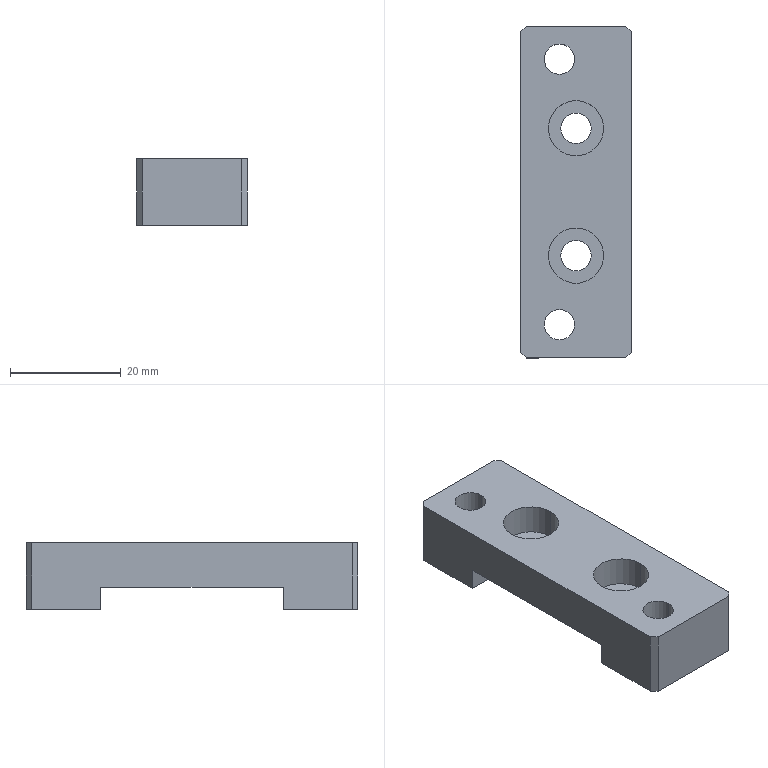Part | SolidWorks | features BaseBody 1 | 1 solid | 34 faces | box 20 x 60 x 12 mm | volume 9580 mm3 | plane 18 | cylinder 16 | commonest cylinder face diameters 5.5 x8 10 x8
STEP:
#1=CARTESIAN_POINT('',(93.009,112.551,12.));
#2=VERTEX_POINT('',#1);
#3=CARTESIAN_POINT('',(87.509,112.551,12.));
#4=VERTEX_POINT('',#3);
#5=CARTESIAN_POINT('',(90.259,112.551,12.));
#6=DIRECTION('',(0.,0.,-1.));
#7=DIRECTION('',(-1.,0.,0.));
#8=AXIS2_PLACEMENT_3D('',#5,#6,#7);
#9=CIRCLE('',#8,2.75);
#10=EDGE_CURVE('',#2,#4,#9,.T.);
#11=ORIENTED_EDGE('',*,*,#10,.F.);
#12=CARTESIAN_POINT('',(93.009,112.551,5.5));
#13=VERTEX_POINT('',#12);
#14=CARTESIAN_POINT('',(93.009,112.551,64.374));
#15=DIRECTION('',(0.,0.,-1.));
#16=VECTOR('',#15,1000.);
#17=LINE('',#14,#16);
#18=EDGE_CURVE('',#2,#13,#17,.T.);
#19=ORIENTED_EDGE('',*,*,#18,.T.);
#20=CARTESIAN_POINT('',(87.509,112.551,5.5));
#21=VERTEX_POINT('',#20);
#22=CARTESIAN_POINT('',(90.259,112.551,5.5));
#23=DIRECTION('',(0.,0.,1.));
#24=DIRECTION('',(-1.,0.,0.));
#25=AXIS2_PLACEMENT_3D('',#22,#23,#24);
#26=CIRCLE('',#25,2.75);
#27=EDGE_CURVE('',#21,#13,#26,.T.);
#28=ORIENTED_EDGE('',*,*,#27,.F.);
#29=CARTESIAN_POINT('',(87.509,112.551,64.374));
#30=DIRECTION('',(0.,0.,-1.));
#31=VECTOR('',#30,1000.);
#32=LINE('',#29,#31);
#33=EDGE_CURVE('',#4,#21,#32,.T.);
#34=ORIENTED_EDGE('',*,*,#33,.F.);
#35=EDGE_LOOP('',(#11,#19,#28,#34));
#36=FACE_OUTER_BOUND('',#35,.T.);
#37=CARTESIAN_POINT('',(90.259,112.551,64.374));
#38=DIRECTION('',(0.,0.,-1.));
#39=DIRECTION('',(-1.,0.,0.));
#40=AXIS2_PLACEMENT_3D('',#37,#38,#39);
#41=CYLINDRICAL_SURFACE('',#40,2.75);
#42=ADVANCED_FACE('',(#36),#41,.F.);
#43=CARTESIAN_POINT('',(93.009,64.551,12.));
#44=VERTEX_POINT('',#43);
#45=CARTESIAN_POINT('',(87.509,64.551,12.));
#46=VERTEX_POINT('',#45);
#47=CARTESIAN_POINT('',(90.259,64.551,12.));
#48=DIRECTION('',(0.,0.,-1.));
#49=DIRECTION('',(-1.,0.,0.));
#50=AXIS2_PLACEMENT_3D('',#47,#48,#49);
#51=CIRCLE('',#50,2.75);
#52=EDGE_CURVE('',#44,#46,#51,.T.);
#53=ORIENTED_EDGE('',*,*,#52,.F.);
#54=CARTESIAN_POINT('',(93.009,64.551,5.5));
#55=VERTEX_POINT('',#54);
#56=CARTESIAN_POINT('',(93.009,64.551,64.374));
#57=DIRECTION('',(0.,0.,-1.));
#58=VECTOR('',#57,1000.);
#59=LINE('',#56,#58);
#60=EDGE_CURVE('',#44,#55,#59,.T.);
#61=ORIENTED_EDGE('',*,*,#60,.T.);
#62=CARTESIAN_POINT('',(87.509,64.551,5.5));
#63=VERTEX_POINT('',#62);
#64=CARTESIAN_POINT('',(90.259,64.551,5.5));
#65=DIRECTION('',(0.,0.,1.));
#66=DIRECTION('',(-1.,0.,0.));
#67=AXIS2_PLACEMENT_3D('',#64,#65,#66);
#68=CIRCLE('',#67,2.75);
#69=EDGE_CURVE('',#63,#55,#68,.T.);
#70=ORIENTED_EDGE('',*,*,#69,.F.);
#71=CARTESIAN_POINT('',(87.509,64.551,64.374));
#72=DIRECTION('',(0.,0.,-1.));
#73=VECTOR('',#72,1000.);
#74=LINE('',#71,#73);
#75=EDGE_CURVE('',#46,#63,#74,.T.);
#76=ORIENTED_EDGE('',*,*,#75,.F.);
#77=EDGE_LOOP('',(#53,#61,#70,#76));
#78=FACE_OUTER_BOUND('',#77,.T.);
#79=CARTESIAN_POINT('',(90.259,64.551,64.374));
#80=DIRECTION('',(0.,0.,-1.));
#81=DIRECTION('',(-1.,0.,0.));
#82=AXIS2_PLACEMENT_3D('',#79,#80,#81);
#83=CYLINDRICAL_SURFACE('',#82,2.75);
#84=ADVANCED_FACE('',(#78),#83,.F.);
#85=CARTESIAN_POINT('',(88.259,100.051,6.5));
#86=VERTEX_POINT('',#85);
#87=CARTESIAN_POINT('',(98.259,100.051,6.5));
#88=VERTEX_POINT('',#87);
#89=CARTESIAN_POINT('',(93.259,100.051,6.5));
#90=DIRECTION('',(0.,0.,1.));
#91=DIRECTION('',(1.,0.,0.));
#92=AXIS2_PLACEMENT_3D('',#89,#90,#91);
#93=CIRCLE('',#92,5.);
#94=EDGE_CURVE('',#86,#88,#93,.T.);
#95=ORIENTED_EDGE('',*,*,#94,.F.);
#96=CARTESIAN_POINT('',(88.259,100.051,12.));
#97=VERTEX_POINT('',#96);
#98=CARTESIAN_POINT('',(88.259,100.051,9.25));
#99=DIRECTION('',(0.,0.,1.));
#100=VECTOR('',#99,1000.);
#101=LINE('',#98,#100);
#102=EDGE_CURVE('',#86,#97,#101,.T.);
#103=ORIENTED_EDGE('',*,*,#102,.T.);
#104=CARTESIAN_POINT('',(98.259,100.051,12.));
#105=VERTEX_POINT('',#104);
#106=CARTESIAN_POINT('',(93.259,100.051,12.));
#107=DIRECTION('',(0.,0.,-1.));
#108=DIRECTION('',(1.,0.,0.));
#109=AXIS2_PLACEMENT_3D('',#106,#107,#108);
#110=CIRCLE('',#109,5.);
#111=EDGE_CURVE('',#105,#97,#110,.T.);
#112=ORIENTED_EDGE('',*,*,#111,.F.);
#113=CARTESIAN_POINT('',(98.259,100.051,9.25));
#114=DIRECTION('',(0.,0.,1.));
#115=VECTOR('',#114,1000.);
#116=LINE('',#113,#115);
#117=EDGE_CURVE('',#88,#105,#116,.T.);
#118=ORIENTED_EDGE('',*,*,#117,.F.);
#119=EDGE_LOOP('',(#95,#103,#112,#118));
#120=FACE_OUTER_BOUND('',#119,.T.);
#121=CARTESIAN_POINT('',(93.259,100.051,9.25));
#122=DIRECTION('',(0.,0.,1.));
#123=DIRECTION('',(1.,0.,0.));
#124=AXIS2_PLACEMENT_3D('',#121,#122,#123);
#125=CYLINDRICAL_SURFACE('',#124,5.);
#126=ADVANCED_FACE('',(#120),#125,.F.);
#127=CARTESIAN_POINT('',(88.259,77.051,6.5));
#128=VERTEX_POINT('',#127);
#129=CARTESIAN_POINT('',(98.259,77.051,6.5));
#130=VERTEX_POINT('',#129);
#131=CARTESIAN_POINT('',(93.259,77.051,6.5));
#132=DIRECTION('',(0.,0.,1.));
#133=DIRECTION('',(1.,0.,0.));
#134=AXIS2_PLACEMENT_3D('',#131,#132,#133);
#135=CIRCLE('',#134,5.);
#136=EDGE_CURVE('',#128,#130,#135,.T.);
#137=ORIENTED_EDGE('',*,*,#136,.F.);
#138=CARTESIAN_POINT('',(88.259,77.051,12.));
#139=VERTEX_POINT('',#138);
#140=CARTESIAN_POINT('',(88.259,77.051,9.25));
#141=DIRECTION('',(0.,0.,1.));
#142=VECTOR('',#141,1000.);
#143=LINE('',#140,#142);
#144=EDGE_CURVE('',#128,#139,#143,.T.);
#145=ORIENTED_EDGE('',*,*,#144,.T.);
#146=CARTESIAN_POINT('',(98.259,77.051,12.));
#147=VERTEX_POINT('',#146);
#148=CARTESIAN_POINT('',(93.259,77.051,12.));
#149=DIRECTION('',(0.,0.,-1.));
#150=DIRECTION('',(1.,0.,0.));
#151=AXIS2_PLACEMENT_3D('',#148,#149,#150);
#152=CIRCLE('',#151,5.);
#153=EDGE_CURVE('',#147,#139,#152,.T.);
#154=ORIENTED_EDGE('',*,*,#153,.F.);
#155=CARTESIAN_POINT('',(98.259,77.051,9.25));
#156=DIRECTION('',(0.,0.,1.));
#157=VECTOR('',#156,1000.);
#158=LINE('',#155,#157);
#159=EDGE_CURVE('',#130,#147,#158,.T.);
#160=ORIENTED_EDGE('',*,*,#159,.F.);
#161=EDGE_LOOP('',(#137,#145,#154,#160));
#162=FACE_OUTER_BOUND('',#161,.T.);
#163=CARTESIAN_POINT('',(93.259,77.051,9.25));
#164=DIRECTION('',(0.,0.,1.));
#165=DIRECTION('',(1.,0.,0.));
#166=AXIS2_PLACEMENT_3D('',#163,#164,#165);
#167=CYLINDRICAL_SURFACE('',#166,5.);
#168=ADVANCED_FACE('',(#162),#167,.F.);
#169=CARTESIAN_POINT('',(95.259,112.551,5.5));
#170=VERTEX_POINT('',#169);
#171=CARTESIAN_POINT('',(85.259,112.551,5.5));
#172=VERTEX_POINT('',#171);
#173=CARTESIAN_POINT('',(90.259,112.551,5.5));
#174=DIRECTION('',(0.,0.,-1.));
#175=DIRECTION('',(-1.,0.,0.));
#176=AXIS2_PLACEMENT_3D('',#173,#174,#175);
#177=CIRCLE('',#176,5.);
#178=EDGE_CURVE('',#170,#172,#177,.T.);
#179=ORIENTED_EDGE('',*,*,#178,.F.);
#180=CARTESIAN_POINT('',(95.259,112.551,0.));
#181=VERTEX_POINT('',#180);
#182=CARTESIAN_POINT('',(95.259,112.551,2.75));
#183=DIRECTION('',(0.,0.,-1.));
#184=VECTOR('',#183,1000.);
#185=LINE('',#182,#184);
#186=EDGE_CURVE('',#170,#181,#185,.T.);
#187=ORIENTED_EDGE('',*,*,#186,.T.);
#188=CARTESIAN_POINT('',(85.259,112.551,0.));
#189=VERTEX_POINT('',#188);
#190=CARTESIAN_POINT('',(90.259,112.551,0.));
#191=DIRECTION('',(0.,0.,-1.));
#192=DIRECTION('',(-1.,0.,0.));
#193=AXIS2_PLACEMENT_3D('',#190,#191,#192);
#194=CIRCLE('',#193,5.);
#195=EDGE_CURVE('',#181,#189,#194,.T.);
#196=ORIENTED_EDGE('',*,*,#195,.T.);
#197=CARTESIAN_POINT('',(85.259,112.551,2.75));
#198=DIRECTION('',(0.,0.,-1.));
#199=VECTOR('',#198,1000.);
#200=LINE('',#197,#199);
#201=EDGE_CURVE('',#172,#189,#200,.T.);
#202=ORIENTED_EDGE('',*,*,#201,.F.);
#203=EDGE_LOOP('',(#179,#187,#196,#202));
#204=FACE_OUTER_BOUND('',#203,.T.);
#205=CARTESIAN_POINT('',(90.259,112.551,2.75));
#206=DIRECTION('',(0.,0.,-1.));
#207=DIRECTION('',(-1.,0.,0.));
#208=AXIS2_PLACEMENT_3D('',#205,#206,#207);
#209=CYLINDRICAL_SURFACE('',#208,5.);
#210=ADVANCED_FACE('',(#204),#209,.F.);
#211=CARTESIAN_POINT('',(95.259,64.551,5.5));
#212=VERTEX_POINT('',#211);
#213=CARTESIAN_POINT('',(85.259,64.551,5.5));
#214=VERTEX_POINT('',#213);
#215=CARTESIAN_POINT('',(90.259,64.551,5.5));
#216=DIRECTION('',(0.,0.,-1.));
#217=DIRECTION('',(-1.,0.,0.));
#218=AXIS2_PLACEMENT_3D('',#215,#216,#217);
#219=CIRCLE('',#218,5.);
#220=EDGE_CURVE('',#212,#214,#219,.T.);
#221=ORIENTED_EDGE('',*,*,#220,.F.);
#222=CARTESIAN_POINT('',(95.259,64.551,0.));
#223=VERTEX_POINT('',#222);
#224=CARTESIAN_POINT('',(95.259,64.551,2.75));
#225=DIRECTION('',(0.,0.,-1.));
#226=VECTOR('',#225,1000.);
#227=LINE('',#224,#226);
#228=EDGE_CURVE('',#212,#223,#227,.T.);
#229=ORIENTED_EDGE('',*,*,#228,.T.);
#230=CARTESIAN_POINT('',(85.259,64.551,0.));
#231=VERTEX_POINT('',#230);
#232=CARTESIAN_POINT('',(90.259,64.551,0.));
#233=DIRECTION('',(0.,0.,-1.));
#234=DIRECTION('',(-1.,0.,0.));
#235=AXIS2_PLACEMENT_3D('',#232,#233,#234);
#236=CIRCLE('',#235,5.);
#237=EDGE_CURVE('',#223,#231,#236,.T.);
#238=ORIENTED_EDGE('',*,*,#237,.T.);
#239=CARTESIAN_POINT('',(85.259,64.551,2.75));
#240=DIRECTION('',(0.,0.,-1.));
#241=VECTOR('',#240,1000.);
#242=LINE('',#239,#241);
#243=EDGE_CURVE('',#214,#231,#242,.T.);
#244=ORIENTED_EDGE('',*,*,#243,.F.);
#245=EDGE_LOOP('',(#221,#229,#238,#244));
#246=FACE_OUTER_BOUND('',#245,.T.);
#247=CARTESIAN_POINT('',(90.259,64.551,2.75));
#248=DIRECTION('',(0.,0.,-1.));
#249=DIRECTION('',(-1.,0.,0.));
#250=AXIS2_PLACEMENT_3D('',#247,#248,#249);
#251=CYLINDRICAL_SURFACE('',#250,5.);
#252=ADVANCED_FACE('',(#246),#251,.F.);
#253=CARTESIAN_POINT('',(96.009,100.051,4.));
#254=VERTEX_POINT('',#253);
#255=CARTESIAN_POINT('',(90.509,100.051,4.));
#256=VERTEX_POINT('',#255);
#257=CARTESIAN_POINT('',(93.259,100.051,4.));
#258=DIRECTION('',(0.,0.,-1.));
#259=DIRECTION('',(1.,0.,0.));
#260=AXIS2_PLACEMENT_3D('',#257,#258,#259);
#261=CIRCLE('',#260,2.75);
#262=EDGE_CURVE('',#254,#256,#261,.T.);
#263=ORIENTED_EDGE('',*,*,#262,.T.);
#264=CARTESIAN_POINT('',(90.509,100.051,6.5));
#265=VERTEX_POINT('',#264);
#266=CARTESIAN_POINT('',(90.509,100.051,-52.374));
#267=DIRECTION('',(0.,0.,1.));
#268=VECTOR('',#267,1000.);
#269=LINE('',#266,#268);
#270=EDGE_CURVE('',#256,#265,#269,.T.);
#271=ORIENTED_EDGE('',*,*,#270,.T.);
#272=CARTESIAN_POINT('',(96.009,100.051,6.5));
#273=VERTEX_POINT('',#272);
#274=CARTESIAN_POINT('',(93.259,100.051,6.5));
#275=DIRECTION('',(0.,0.,-1.));
#276=DIRECTION('',(1.,0.,0.));
#277=AXIS2_PLACEMENT_3D('',#274,#275,#276);
#278=CIRCLE('',#277,2.75);
#279=EDGE_CURVE('',#273,#265,#278,.T.);
#280=ORIENTED_EDGE('',*,*,#279,.F.);
#281=CARTESIAN_POINT('',(96.009,100.051,-52.374));
#282=DIRECTION('',(0.,0.,1.));
#283=VECTOR('',#282,1000.);
#284=LINE('',#281,#283);
#285=EDGE_CURVE('',#254,#273,#284,.T.);
#286=ORIENTED_EDGE('',*,*,#285,.F.);
#287=EDGE_LOOP('',(#263,#271,#280,#286));
#288=FACE_OUTER_BOUND('',#287,.T.);
#289=CARTESIAN_POINT('',(93.259,100.051,-52.374));
#290=DIRECTION('',(0.,0.,1.));
#291=DIRECTION('',(1.,0.,0.));
#292=AXIS2_PLACEMENT_3D('',#289,#290,#291);
#293=CYLINDRICAL_SURFACE('',#292,2.75);
#294=ADVANCED_FACE('',(#288),#293,.F.);
#295=CARTESIAN_POINT('',(96.009,77.051,4.));
#296=VERTEX_POINT('',#295);
#297=CARTESIAN_POINT('',(90.509,77.051,4.));
#298=VERTEX_POINT('',#297);
#299=CARTESIAN_POINT('',(93.259,77.051,4.));
#300=DIRECTION('',(0.,0.,-1.));
#301=DIRECTION('',(1.,0.,0.));
#302=AXIS2_PLACEMENT_3D('',#299,#300,#301);
#303=CIRCLE('',#302,2.75);
#304=EDGE_CURVE('',#296,#298,#303,.T.);
#305=ORIENTED_EDGE('',*,*,#304,.T.);
#306=CARTESIAN_POINT('',(90.509,77.051,6.5));
#307=VERTEX_POINT('',#306);
#308=CARTESIAN_POINT('',(90.509,77.051,-52.374));
#309=DIRECTION('',(0.,0.,1.));
#310=VECTOR('',#309,1000.);
#311=LINE('',#308,#310);
#312=EDGE_CURVE('',#298,#307,#311,.T.);
#313=ORIENTED_EDGE('',*,*,#312,.T.);
#314=CARTESIAN_POINT('',(96.009,77.051,6.5));
#315=VERTEX_POINT('',#314);
#316=CARTESIAN_POINT('',(93.259,77.051,6.5));
#317=DIRECTION('',(0.,0.,-1.));
#318=DIRECTION('',(1.,0.,0.));
#319=AXIS2_PLACEMENT_3D('',#316,#317,#318);
#320=CIRCLE('',#319,2.75);
#321=EDGE_CURVE('',#315,#307,#320,.T.);
#322=ORIENTED_EDGE('',*,*,#321,.F.);
#323=CARTESIAN_POINT('',(96.009,77.051,-52.374));
#324=DIRECTION('',(0.,0.,1.));
#325=VECTOR('',#324,1000.);
#326=LINE('',#323,#325);
#327=EDGE_CURVE('',#296,#315,#326,.T.);
#328=ORIENTED_EDGE('',*,*,#327,.F.);
#329=EDGE_LOOP('',(#305,#313,#322,#328));
#330=FACE_OUTER_BOUND('',#329,.T.);
#331=CARTESIAN_POINT('',(93.259,77.051,-52.374));
#332=DIRECTION('',(0.,0.,1.));
#333=DIRECTION('',(1.,0.,0.));
#334=AXIS2_PLACEMENT_3D('',#331,#332,#333);
#335=CYLINDRICAL_SURFACE('',#334,2.75);
#336=ADVANCED_FACE('',(#330),#335,.F.);
#337=CARTESIAN_POINT('',(90.259,112.551,12.));
#338=DIRECTION('',(0.,0.,-1.));
#339=DIRECTION('',(-1.,0.,0.));
#340=AXIS2_PLACEMENT_3D('',#337,#338,#339);
#341=CIRCLE('',#340,2.75);
#342=EDGE_CURVE('',#4,#2,#341,.T.);
#343=ORIENTED_EDGE('',*,*,#342,.T.);
#344=ORIENTED_EDGE('',*,*,#10,.T.);
#345=EDGE_LOOP('',(#343,#344));
#346=FACE_BOUND('',#345,.T.);
#347=CARTESIAN_POINT('',(90.259,64.551,12.));
#348=DIRECTION('',(0.,0.,-1.));
#349=DIRECTION('',(-1.,0.,0.));
#350=AXIS2_PLACEMENT_3D('',#347,#348,#349);
#351=CIRCLE('',#350,2.75);
#352=EDGE_CURVE('',#46,#44,#351,.T.);
#353=ORIENTED_EDGE('',*,*,#352,.T.);
#354=ORIENTED_EDGE('',*,*,#52,.T.);
#355=EDGE_LOOP('',(#353,#354));
#356=FACE_BOUND('',#355,.T.);
#357=ORIENTED_EDGE('',*,*,#111,.T.);
#358=CARTESIAN_POINT('',(93.259,100.051,12.));
#359=DIRECTION('',(0.,0.,-1.));
#360=DIRECTION('',(1.,0.,0.));
#361=AXIS2_PLACEMENT_3D('',#358,#359,#360);
#362=CIRCLE('',#361,5.);
#363=EDGE_CURVE('',#97,#105,#362,.T.);
#364=ORIENTED_EDGE('',*,*,#363,.T.);
#365=EDGE_LOOP('',(#357,#364));
#366=FACE_BOUND('',#365,.T.);
#367=ORIENTED_EDGE('',*,*,#153,.T.);
#368=CARTESIAN_POINT('',(93.259,77.051,12.));
#369=DIRECTION('',(0.,0.,-1.));
#370=DIRECTION('',(1.,0.,0.));
#371=AXIS2_PLACEMENT_3D('',#368,#369,#370);
#372=CIRCLE('',#371,5.);
#373=EDGE_CURVE('',#139,#147,#372,.T.);
#374=ORIENTED_EDGE('',*,*,#373,.T.);
#375=EDGE_LOOP('',(#367,#374));
#376=FACE_BOUND('',#375,.T.);
#377=CARTESIAN_POINT('',(84.259,58.551,12.));
#378=VERTEX_POINT('',#377);
#379=CARTESIAN_POINT('',(83.259,59.551,12.));
#380=VERTEX_POINT('',#379);
#381=CARTESIAN_POINT('',(83.759,59.051,12.));
#382=DIRECTION('',(-0.7071,0.7071,0.));
#383=VECTOR('',#382,1000.);
#384=LINE('',#381,#383);
#385=EDGE_CURVE('',#378,#380,#384,.T.);
#386=ORIENTED_EDGE('',*,*,#385,.F.);
#387=CARTESIAN_POINT('',(102.259,58.551,12.));
#388=VERTEX_POINT('',#387);
#389=CARTESIAN_POINT('',(93.259,58.551,12.));
#390=DIRECTION('',(1.,0.,0.));
#391=VECTOR('',#390,1000.);
#392=LINE('',#389,#391);
#393=EDGE_CURVE('',#378,#388,#392,.T.);
#394=ORIENTED_EDGE('',*,*,#393,.T.);
#395=CARTESIAN_POINT('',(103.259,59.551,12.));
#396=VERTEX_POINT('',#395);
#397=CARTESIAN_POINT('',(102.759,59.051,12.));
#398=DIRECTION('',(-0.7071,-0.7071,0.));
#399=VECTOR('',#398,1000.);
#400=LINE('',#397,#399);
#401=EDGE_CURVE('',#396,#388,#400,.T.);
#402=ORIENTED_EDGE('',*,*,#401,.F.);
#403=CARTESIAN_POINT('',(103.259,117.551,12.));
#404=VERTEX_POINT('',#403);
#405=CARTESIAN_POINT('',(103.259,88.551,12.));
#406=DIRECTION('',(0.,1.,0.));
#407=VECTOR('',#406,1000.);
#408=LINE('',#405,#407);
#409=EDGE_CURVE('',#396,#404,#408,.T.);
#410=ORIENTED_EDGE('',*,*,#409,.T.);
#411=CARTESIAN_POINT('',(102.259,118.551,12.));
#412=VERTEX_POINT('',#411);
#413=CARTESIAN_POINT('',(102.759,118.051,12.));
#414=DIRECTION('',(0.7071,-0.7071,0.));
#415=VECTOR('',#414,1000.);
#416=LINE('',#413,#415);
#417=EDGE_CURVE('',#412,#404,#416,.T.);
#418=ORIENTED_EDGE('',*,*,#417,.F.);
#419=CARTESIAN_POINT('',(84.259,118.551,12.));
#420=VERTEX_POINT('',#419);
#421=CARTESIAN_POINT('',(93.259,118.551,12.));
#422=DIRECTION('',(-1.,0.,0.));
#423=VECTOR('',#422,1000.);
#424=LINE('',#421,#423);
#425=EDGE_CURVE('',#412,#420,#424,.T.);
#426=ORIENTED_EDGE('',*,*,#425,.T.);
#427=CARTESIAN_POINT('',(83.259,117.551,12.));
#428=VERTEX_POINT('',#427);
#429=CARTESIAN_POINT('',(83.759,118.051,12.));
#430=DIRECTION('',(0.7071,0.7071,0.));
#431=VECTOR('',#430,1000.);
#432=LINE('',#429,#431);
#433=EDGE_CURVE('',#428,#420,#432,.T.);
#434=ORIENTED_EDGE('',*,*,#433,.F.);
#435=CARTESIAN_POINT('',(83.259,88.551,12.));
#436=DIRECTION('',(0.,-1.,0.));
#437=VECTOR('',#436,1000.);
#438=LINE('',#435,#437);
#439=EDGE_CURVE('',#428,#380,#438,.T.);
#440=ORIENTED_EDGE('',*,*,#439,.T.);
#441=EDGE_LOOP('',(#386,#394,#402,#410,#418,#426,#434,#440));
#442=FACE_OUTER_BOUND('',#441,.T.);
#443=CARTESIAN_POINT('',(93.259,88.551,12.));
#444=DIRECTION('',(0.,0.,1.));
#445=DIRECTION('',(1.,0.,0.));
#446=AXIS2_PLACEMENT_3D('',#443,#444,#445);
#447=PLANE('',#446);
#448=ADVANCED_FACE('',(#346,#356,#366,#376,#442),#447,.T.);
#449=ORIENTED_EDGE('',*,*,#18,.F.);
#450=ORIENTED_EDGE('',*,*,#342,.F.);
#451=ORIENTED_EDGE('',*,*,#33,.T.);
#452=CARTESIAN_POINT('',(90.259,112.551,5.5));
#453=DIRECTION('',(0.,0.,1.));
#454=DIRECTION('',(-1.,0.,0.));
#455=AXIS2_PLACEMENT_3D('',#452,#453,#454);
#456=CIRCLE('',#455,2.75);
#457=EDGE_CURVE('',#13,#21,#456,.T.);
#458=ORIENTED_EDGE('',*,*,#457,.F.);
#459=EDGE_LOOP('',(#449,#450,#451,#458));
#460=FACE_OUTER_BOUND('',#459,.T.);
#461=CARTESIAN_POINT('',(90.259,112.551,64.374));
#462=DIRECTION('',(0.,0.,-1.));
#463=DIRECTION('',(-1.,0.,0.));
#464=AXIS2_PLACEMENT_3D('',#461,#462,#463);
#465=CYLINDRICAL_SURFACE('',#464,2.75);
#466=ADVANCED_FACE('',(#460),#465,.F.);
#467=ORIENTED_EDGE('',*,*,#60,.F.);
#468=ORIENTED_EDGE('',*,*,#352,.F.);
#469=ORIENTED_EDGE('',*,*,#75,.T.);
#470=CARTESIAN_POINT('',(90.259,64.551,5.5));
#471=DIRECTION('',(0.,0.,1.));
#472=DIRECTION('',(-1.,0.,0.));
#473=AXIS2_PLACEMENT_3D('',#470,#471,#472);
#474=CIRCLE('',#473,2.75);
#475=EDGE_CURVE('',#55,#63,#474,.T.);
#476=ORIENTED_EDGE('',*,*,#475,.F.);
#477=EDGE_LOOP('',(#467,#468,#469,#476));
#478=FACE_OUTER_BOUND('',#477,.T.);
#479=CARTESIAN_POINT('',(90.259,64.551,64.374));
#480=DIRECTION('',(0.,0.,-1.));
#481=DIRECTION('',(-1.,0.,0.));
#482=AXIS2_PLACEMENT_3D('',#479,#480,#481);
#483=CYLINDRICAL_SURFACE('',#482,2.75);
#484=ADVANCED_FACE('',(#478),#483,.F.);
#485=ORIENTED_EDGE('',*,*,#102,.F.);
#486=CARTESIAN_POINT('',(93.259,100.051,6.5));
#487=DIRECTION('',(0.,0.,1.));
#488=DIRECTION('',(1.,0.,0.));
#489=AXIS2_PLACEMENT_3D('',#486,#487,#488);
#490=CIRCLE('',#489,5.);
#491=EDGE_CURVE('',#88,#86,#490,.T.);
#492=ORIENTED_EDGE('',*,*,#491,.F.);
#493=ORIENTED_EDGE('',*,*,#117,.T.);
#494=ORIENTED_EDGE('',*,*,#363,.F.);
#495=EDGE_LOOP('',(#485,#492,#493,#494));
#496=FACE_OUTER_BOUND('',#495,.T.);
#497=CARTESIAN_POINT('',(93.259,100.051,9.25));
#498=DIRECTION('',(0.,0.,1.));
#499=DIRECTION('',(1.,0.,0.));
#500=AXIS2_PLACEMENT_3D('',#497,#498,#499);
#501=CYLINDRICAL_SURFACE('',#500,5.);
#502=ADVANCED_FACE('',(#496),#501,.F.);
#503=ORIENTED_EDGE('',*,*,#144,.F.);
#504=CARTESIAN_POINT('',(93.259,77.051,6.5));
#505=DIRECTION('',(0.,0.,1.));
#506=DIRECTION('',(1.,0.,0.));
#507=AXIS2_PLACEMENT_3D('',#504,#505,#506);
#508=CIRCLE('',#507,5.);
#509=EDGE_CURVE('',#130,#128,#508,.T.);
#510=ORIENTED_EDGE('',*,*,#509,.F.);
#511=ORIENTED_EDGE('',*,*,#159,.T.);
#512=ORIENTED_EDGE('',*,*,#373,.F.);
#513=EDGE_LOOP('',(#503,#510,#511,#512));
#514=FACE_OUTER_BOUND('',#513,.T.);
#515=CARTESIAN_POINT('',(93.259,77.051,9.25));
#516=DIRECTION('',(0.,0.,1.));
#517=DIRECTION('',(1.,0.,0.));
#518=AXIS2_PLACEMENT_3D('',#515,#516,#517);
#519=CYLINDRICAL_SURFACE('',#518,5.);
#520=ADVANCED_FACE('',(#514),#519,.F.);
#521=CARTESIAN_POINT('',(84.259,58.551,0.));
#522=VERTEX_POINT('',#521);
#523=CARTESIAN_POINT('',(84.259,58.551,0.));
#524=DIRECTION('',(0.,0.,-1.));
#525=VECTOR('',#524,1000.);
#526=LINE('',#523,#525);
#527=EDGE_CURVE('',#378,#522,#526,.T.);
#528=ORIENTED_EDGE('',*,*,#527,.T.);
#529=CARTESIAN_POINT('',(102.259,58.551,0.));
#530=VERTEX_POINT('',#529);
#531=CARTESIAN_POINT('',(103.259,58.551,0.));
#532=DIRECTION('',(1.,0.,0.));
#533=VECTOR('',#532,1000.);
#534=LINE('',#531,#533);
#535=EDGE_CURVE('',#522,#530,#534,.T.);
#536=ORIENTED_EDGE('',*,*,#535,.T.);
#537=CARTESIAN_POINT('',(102.259,58.551,0.));
#538=DIRECTION('',(0.,0.,1.));
#539=VECTOR('',#538,1000.);
#540=LINE('',#537,#539);
#541=EDGE_CURVE('',#530,#388,#540,.T.);
#542=ORIENTED_EDGE('',*,*,#541,.T.);
#543=ORIENTED_EDGE('',*,*,#393,.F.);
#544=EDGE_LOOP('',(#528,#536,#542,#543));
#545=FACE_OUTER_BOUND('',#544,.T.);
#546=CARTESIAN_POINT('',(103.259,58.551,0.));
#547=DIRECTION('',(0.,-1.,0.));
#548=DIRECTION('',(0.,0.,-1.));
#549=AXIS2_PLACEMENT_3D('',#546,#547,#548);
#550=PLANE('',#549);
#551=ADVANCED_FACE('',(#545),#550,.T.);
#552=CARTESIAN_POINT('',(83.259,72.051,4.));
#553=VERTEX_POINT('',#552);
#554=CARTESIAN_POINT('',(83.259,72.051,0.));
#555=VERTEX_POINT('',#554);
#556=CARTESIAN_POINT('',(83.259,72.051,0.));
#557=DIRECTION('',(0.,0.,-1.));
#558=VECTOR('',#557,1000.);
#559=LINE('',#556,#558);
#560=EDGE_CURVE('',#553,#555,#559,.T.);
#561=ORIENTED_EDGE('',*,*,#560,.T.);
#562=CARTESIAN_POINT('',(83.259,59.551,0.));
#563=VERTEX_POINT('',#562);
#564=CARTESIAN_POINT('',(83.259,58.551,0.));
#565=DIRECTION('',(0.,-1.,0.));
#566=VECTOR('',#565,1000.);
#567=LINE('',#564,#566);
#568=EDGE_CURVE('',#555,#563,#567,.T.);
#569=ORIENTED_EDGE('',*,*,#568,.T.);
#570=CARTESIAN_POINT('',(83.259,59.551,0.));
#571=DIRECTION('',(0.,0.,1.));
#572=VECTOR('',#571,1000.);
#573=LINE('',#570,#572);
#574=EDGE_CURVE('',#563,#380,#573,.T.);
#575=ORIENTED_EDGE('',*,*,#574,.T.);
#576=ORIENTED_EDGE('',*,*,#439,.F.);
#577=CARTESIAN_POINT('',(83.259,117.551,0.));
#578=VERTEX_POINT('',#577);
#579=CARTESIAN_POINT('',(83.259,117.551,0.));
#580=DIRECTION('',(0.,0.,-1.));
#581=VECTOR('',#580,1000.);
#582=LINE('',#579,#581);
#583=EDGE_CURVE('',#428,#578,#582,.T.);
#584=ORIENTED_EDGE('',*,*,#583,.T.);
#585=CARTESIAN_POINT('',(83.259,105.051,0.));
#586=VERTEX_POINT('',#585);
#587=CARTESIAN_POINT('',(83.259,58.551,0.));
#588=DIRECTION('',(0.,-1.,0.));
#589=VECTOR('',#588,1000.);
#590=LINE('',#587,#589);
#591=EDGE_CURVE('',#578,#586,#590,.T.);
#592=ORIENTED_EDGE('',*,*,#591,.T.);
#593=CARTESIAN_POINT('',(83.259,105.051,4.));
#594=VERTEX_POINT('',#593);
#595=CARTESIAN_POINT('',(83.259,105.051,0.));
#596=DIRECTION('',(0.,0.,1.));
#597=VECTOR('',#596,1000.);
#598=LINE('',#595,#597);
#599=EDGE_CURVE('',#586,#594,#598,.T.);
#600=ORIENTED_EDGE('',*,*,#599,.T.);
#601=CARTESIAN_POINT('',(83.259,58.551,4.));
#602=DIRECTION('',(0.,-1.,0.));
#603=VECTOR('',#602,1000.);
#604=LINE('',#601,#603);
#605=EDGE_CURVE('',#594,#553,#604,.T.);
#606=ORIENTED_EDGE('',*,*,#605,.T.);
#607=EDGE_LOOP('',(#561,#569,#575,#576,#584,#592,#600,#606));
#608=FACE_OUTER_BOUND('',#607,.T.);
#609=CARTESIAN_POINT('',(83.259,58.551,0.));
#610=DIRECTION('',(-1.,0.,0.));
#611=DIRECTION('',(0.,0.,1.));
#612=AXIS2_PLACEMENT_3D('',#609,#610,#611);
#613=PLANE('',#612);
#614=ADVANCED_FACE('',(#608),#613,.T.);
#615=CARTESIAN_POINT('',(102.259,118.551,0.));
#616=VERTEX_POINT('',#615);
#617=CARTESIAN_POINT('',(102.259,118.551,0.));
#618=DIRECTION('',(0.,0.,-1.));
#619=VECTOR('',#618,1000.);
#620=LINE('',#617,#619);
#621=EDGE_CURVE('',#412,#616,#620,.T.);
#622=ORIENTED_EDGE('',*,*,#621,.T.);
#623=CARTESIAN_POINT('',(84.259,118.551,0.));
#624=VERTEX_POINT('',#623);
#625=CARTESIAN_POINT('',(83.259,118.551,0.));
#626=DIRECTION('',(-1.,0.,0.));
#627=VECTOR('',#626,1000.);
#628=LINE('',#625,#627);
#629=EDGE_CURVE('',#616,#624,#628,.T.);
#630=ORIENTED_EDGE('',*,*,#629,.T.);
#631=CARTESIAN_POINT('',(84.259,118.551,0.));
#632=DIRECTION('',(0.,0.,1.));
#633=VECTOR('',#632,1000.);
#634=LINE('',#631,#633);
#635=EDGE_CURVE('',#624,#420,#634,.T.);
#636=ORIENTED_EDGE('',*,*,#635,.T.);
#637=ORIENTED_EDGE('',*,*,#425,.F.);
#638=EDGE_LOOP('',(#622,#630,#636,#637));
#639=FACE_OUTER_BOUND('',#638,.T.);
#640=CARTESIAN_POINT('',(83.259,118.551,0.));
#641=DIRECTION('',(0.,1.,0.));
#642=DIRECTION('',(0.,0.,1.));
#643=AXIS2_PLACEMENT_3D('',#640,#641,#642);
#644=PLANE('',#643);
#645=ADVANCED_FACE('',(#639),#644,.T.);
#646=CARTESIAN_POINT('',(103.259,117.551,0.));
#647=VERTEX_POINT('',#646);
#648=CARTESIAN_POINT('',(103.259,117.551,0.));
#649=DIRECTION('',(0.,0.,1.));
#650=VECTOR('',#649,1000.);
#651=LINE('',#648,#650);
#652=EDGE_CURVE('',#647,#404,#651,.T.);
#653=ORIENTED_EDGE('',*,*,#652,.T.);
#654=ORIENTED_EDGE('',*,*,#409,.F.);
#655=CARTESIAN_POINT('',(103.259,59.551,0.));
#656=VERTEX_POINT('',#655);
#657=CARTESIAN_POINT('',(103.259,59.551,0.));
#658=DIRECTION('',(0.,0.,-1.));
#659=VECTOR('',#658,1000.);
#660=LINE('',#657,#659);
#661=EDGE_CURVE('',#396,#656,#660,.T.);
#662=ORIENTED_EDGE('',*,*,#661,.T.);
#663=CARTESIAN_POINT('',(103.259,72.051,0.));
#664=VERTEX_POINT('',#663);
#665=CARTESIAN_POINT('',(103.259,118.551,0.));
#666=DIRECTION('',(0.,1.,0.));
#667=VECTOR('',#666,1000.);
#668=LINE('',#665,#667);
#669=EDGE_CURVE('',#656,#664,#668,.T.);
#670=ORIENTED_EDGE('',*,*,#669,.T.);
#671=CARTESIAN_POINT('',(103.259,72.051,4.));
#672=VERTEX_POINT('',#671);
#673=CARTESIAN_POINT('',(103.259,72.051,0.));
#674=DIRECTION('',(0.,0.,1.));
#675=VECTOR('',#674,1000.);
#676=LINE('',#673,#675);
#677=EDGE_CURVE('',#664,#672,#676,.T.);
#678=ORIENTED_EDGE('',*,*,#677,.T.);
#679=CARTESIAN_POINT('',(103.259,105.051,4.));
#680=VERTEX_POINT('',#679);
#681=CARTESIAN_POINT('',(103.259,118.551,4.));
#682=DIRECTION('',(0.,1.,0.));
#683=VECTOR('',#682,1000.);
#684=LINE('',#681,#683);
#685=EDGE_CURVE('',#672,#680,#684,.T.);
#686=ORIENTED_EDGE('',*,*,#685,.T.);
#687=CARTESIAN_POINT('',(103.259,105.051,0.));
#688=VERTEX_POINT('',#687);
#689=CARTESIAN_POINT('',(103.259,105.051,0.));
#690=DIRECTION('',(0.,0.,-1.));
#691=VECTOR('',#690,1000.);
#692=LINE('',#689,#691);
#693=EDGE_CURVE('',#680,#688,#692,.T.);
#694=ORIENTED_EDGE('',*,*,#693,.T.);
#695=CARTESIAN_POINT('',(103.259,118.551,0.));
#696=DIRECTION('',(0.,1.,0.));
#697=VECTOR('',#696,1000.);
#698=LINE('',#695,#697);
#699=EDGE_CURVE('',#688,#647,#698,.T.);
#700=ORIENTED_EDGE('',*,*,#699,.T.);
#701=EDGE_LOOP('',(#653,#654,#662,#670,#678,#686,#694,#700));
#702=FACE_OUTER_BOUND('',#701,.T.);
#703=CARTESIAN_POINT('',(103.259,118.551,0.));
#704=DIRECTION('',(1.,0.,0.));
#705=DIRECTION('',(0.,0.,-1.));
#706=AXIS2_PLACEMENT_3D('',#703,#704,#705);
#707=PLANE('',#706);
#708=ADVANCED_FACE('',(#702),#707,.T.);
#709=ORIENTED_EDGE('',*,*,#27,.T.);
#710=ORIENTED_EDGE('',*,*,#457,.T.);
#711=EDGE_LOOP('',(#709,#710));
#712=FACE_BOUND('',#711,.T.);
#713=CARTESIAN_POINT('',(90.259,112.551,5.5));
#714=DIRECTION('',(0.,0.,-1.));
#715=DIRECTION('',(-1.,0.,0.));
#716=AXIS2_PLACEMENT_3D('',#713,#714,#715);
#717=CIRCLE('',#716,5.);
#718=EDGE_CURVE('',#172,#170,#717,.T.);
#719=ORIENTED_EDGE('',*,*,#718,.T.);
#720=ORIENTED_EDGE('',*,*,#178,.T.);
#721=EDGE_LOOP('',(#719,#720));
#722=FACE_OUTER_BOUND('',#721,.T.);
#723=CARTESIAN_POINT('',(90.259,112.551,5.5));
#724=DIRECTION('',(0.,0.,-1.));
#725=DIRECTION('',(-1.,0.,0.));
#726=AXIS2_PLACEMENT_3D('',#723,#724,#725);
#727=PLANE('',#726);
#728=ADVANCED_FACE('',(#712,#722),#727,.T.);
#729=ORIENTED_EDGE('',*,*,#69,.T.);
#730=ORIENTED_EDGE('',*,*,#475,.T.);
#731=EDGE_LOOP('',(#729,#730));
#732=FACE_BOUND('',#731,.T.);
#733=CARTESIAN_POINT('',(90.259,64.551,5.5));
#734=DIRECTION('',(0.,0.,-1.));
#735=DIRECTION('',(-1.,0.,0.));
#736=AXIS2_PLACEMENT_3D('',#733,#734,#735);
#737=CIRCLE('',#736,5.);
#738=EDGE_CURVE('',#214,#212,#737,.T.);
#739=ORIENTED_EDGE('',*,*,#738,.T.);
#740=ORIENTED_EDGE('',*,*,#220,.T.);
#741=EDGE_LOOP('',(#739,#740));
#742=FACE_OUTER_BOUND('',#741,.T.);
#743=CARTESIAN_POINT('',(90.259,64.551,5.5));
#744=DIRECTION('',(0.,0.,-1.));
#745=DIRECTION('',(-1.,0.,0.));
#746=AXIS2_PLACEMENT_3D('',#743,#744,#745);
#747=PLANE('',#746);
#748=ADVANCED_FACE('',(#732,#742),#747,.T.);
#749=ORIENTED_EDGE('',*,*,#279,.T.);
#750=CARTESIAN_POINT('',(93.259,100.051,6.5));
#751=DIRECTION('',(0.,0.,-1.));
#752=DIRECTION('',(1.,0.,0.));
#753=AXIS2_PLACEMENT_3D('',#750,#751,#752);
#754=CIRCLE('',#753,2.75);
#755=EDGE_CURVE('',#265,#273,#754,.T.);
#756=ORIENTED_EDGE('',*,*,#755,.T.);
#757=EDGE_LOOP('',(#749,#756));
#758=FACE_BOUND('',#757,.T.);
#759=ORIENTED_EDGE('',*,*,#491,.T.);
#760=ORIENTED_EDGE('',*,*,#94,.T.);
#761=EDGE_LOOP('',(#759,#760));
#762=FACE_OUTER_BOUND('',#761,.T.);
#763=CARTESIAN_POINT('',(93.259,100.051,6.5));
#764=DIRECTION('',(0.,0.,1.));
#765=DIRECTION('',(1.,0.,0.));
#766=AXIS2_PLACEMENT_3D('',#763,#764,#765);
#767=PLANE('',#766);
#768=ADVANCED_FACE('',(#758,#762),#767,.T.);
#769=ORIENTED_EDGE('',*,*,#321,.T.);
#770=CARTESIAN_POINT('',(93.259,77.051,6.5));
#771=DIRECTION('',(0.,0.,-1.));
#772=DIRECTION('',(1.,0.,0.));
#773=AXIS2_PLACEMENT_3D('',#770,#771,#772);
#774=CIRCLE('',#773,2.75);
#775=EDGE_CURVE('',#307,#315,#774,.T.);
#776=ORIENTED_EDGE('',*,*,#775,.T.);
#777=EDGE_LOOP('',(#769,#776));
#778=FACE_BOUND('',#777,.T.);
#779=ORIENTED_EDGE('',*,*,#509,.T.);
#780=ORIENTED_EDGE('',*,*,#136,.T.);
#781=EDGE_LOOP('',(#779,#780));
#782=FACE_OUTER_BOUND('',#781,.T.);
#783=CARTESIAN_POINT('',(93.259,77.051,6.5));
#784=DIRECTION('',(0.,0.,1.));
#785=DIRECTION('',(1.,0.,0.));
#786=AXIS2_PLACEMENT_3D('',#783,#784,#785);
#787=PLANE('',#786);
#788=ADVANCED_FACE('',(#778,#782),#787,.T.);
#789=CARTESIAN_POINT('',(90.259,64.551,0.));
#790=DIRECTION('',(0.,0.,-1.));
#791=DIRECTION('',(-1.,0.,0.));
#792=AXIS2_PLACEMENT_3D('',#789,#790,#791);
#793=CIRCLE('',#792,5.);
#794=EDGE_CURVE('',#231,#223,#793,.T.);
#795=ORIENTED_EDGE('',*,*,#794,.F.);
#796=ORIENTED_EDGE('',*,*,#237,.F.);
#797=EDGE_LOOP('',(#795,#796));
#798=FACE_BOUND('',#797,.T.);
#799=ORIENTED_EDGE('',*,*,#535,.F.);
#800=CARTESIAN_POINT('',(83.259,59.551,0.));
#801=DIRECTION('',(0.7071,-0.7071,0.));
#802=VECTOR('',#801,1000.);
#803=LINE('',#800,#802);
#804=EDGE_CURVE('',#563,#522,#803,.T.);
#805=ORIENTED_EDGE('',*,*,#804,.F.);
#806=ORIENTED_EDGE('',*,*,#568,.F.);
#807=CARTESIAN_POINT('',(93.259,72.051,0.));
#808=DIRECTION('',(-1.,0.,0.));
#809=VECTOR('',#808,1000.);
#810=LINE('',#807,#809);
#811=EDGE_CURVE('',#664,#555,#810,.T.);
#812=ORIENTED_EDGE('',*,*,#811,.F.);
#813=ORIENTED_EDGE('',*,*,#669,.F.);
#814=CARTESIAN_POINT('',(102.259,58.551,0.));
#815=DIRECTION('',(0.7071,0.7071,0.));
#816=VECTOR('',#815,1000.);
#817=LINE('',#814,#816);
#818=EDGE_CURVE('',#530,#656,#817,.T.);
#819=ORIENTED_EDGE('',*,*,#818,.F.);
#820=EDGE_LOOP('',(#799,#805,#806,#812,#813,#819));
#821=FACE_OUTER_BOUND('',#820,.T.);
#822=CARTESIAN_POINT('',(93.259,88.551,0.));
#823=DIRECTION('',(0.,0.,1.));
#824=DIRECTION('',(1.,0.,0.));
#825=AXIS2_PLACEMENT_3D('',#822,#823,#824);
#826=PLANE('',#825);
#827=ADVANCED_FACE('',(#798,#821),#826,.F.);
#828=ORIENTED_EDGE('',*,*,#804,.T.);
#829=ORIENTED_EDGE('',*,*,#527,.F.);
#830=ORIENTED_EDGE('',*,*,#385,.T.);
#831=ORIENTED_EDGE('',*,*,#574,.F.);
#832=EDGE_LOOP('',(#828,#829,#830,#831));
#833=FACE_OUTER_BOUND('',#832,.T.);
#834=CARTESIAN_POINT('',(83.759,59.051,0.));
#835=DIRECTION('',(-0.7071,-0.7071,0.));
#836=DIRECTION('',(0.7071,-0.7071,0.));
#837=AXIS2_PLACEMENT_3D('',#834,#835,#836);
#838=PLANE('',#837);
#839=ADVANCED_FACE('',(#833),#838,.T.);
#840=ORIENTED_EDGE('',*,*,#818,.T.);
#841=ORIENTED_EDGE('',*,*,#661,.F.);
#842=ORIENTED_EDGE('',*,*,#401,.T.);
#843=ORIENTED_EDGE('',*,*,#541,.F.);
#844=EDGE_LOOP('',(#840,#841,#842,#843));
#845=FACE_OUTER_BOUND('',#844,.T.);
#846=CARTESIAN_POINT('',(102.759,59.051,0.));
#847=DIRECTION('',(0.7071,-0.7071,0.));
#848=DIRECTION('',(0.7071,0.7071,0.));
#849=AXIS2_PLACEMENT_3D('',#846,#847,#848);
#850=PLANE('',#849);
#851=ADVANCED_FACE('',(#845),#850,.T.);
#852=ORIENTED_EDGE('',*,*,#677,.F.);
#853=ORIENTED_EDGE('',*,*,#811,.T.);
#854=ORIENTED_EDGE('',*,*,#560,.F.);
#855=CARTESIAN_POINT('',(103.259,72.051,4.));
#856=DIRECTION('',(-1.,0.,0.));
#857=VECTOR('',#856,1000.);
#858=LINE('',#855,#857);
#859=EDGE_CURVE('',#672,#553,#858,.T.);
#860=ORIENTED_EDGE('',*,*,#859,.F.);
#861=EDGE_LOOP('',(#852,#853,#854,#860));
#862=FACE_OUTER_BOUND('',#861,.T.);
#863=CARTESIAN_POINT('',(103.259,72.051,0.));
#864=DIRECTION('',(0.,-1.,0.));
#865=DIRECTION('',(0.,0.,-1.));
#866=AXIS2_PLACEMENT_3D('',#863,#864,#865);
#867=PLANE('',#866);
#868=ADVANCED_FACE('',(#862),#867,.F.);
#869=ORIENTED_EDGE('',*,*,#262,.F.);
#870=CARTESIAN_POINT('',(93.259,100.051,4.));
#871=DIRECTION('',(0.,0.,-1.));
#872=DIRECTION('',(1.,0.,0.));
#873=AXIS2_PLACEMENT_3D('',#870,#871,#872);
#874=CIRCLE('',#873,2.75);
#875=EDGE_CURVE('',#256,#254,#874,.T.);
#876=ORIENTED_EDGE('',*,*,#875,.F.);
#877=EDGE_LOOP('',(#869,#876));
#878=FACE_BOUND('',#877,.T.);
#879=ORIENTED_EDGE('',*,*,#304,.F.);
#880=CARTESIAN_POINT('',(93.259,77.051,4.));
#881=DIRECTION('',(0.,0.,-1.));
#882=DIRECTION('',(1.,0.,0.));
#883=AXIS2_PLACEMENT_3D('',#880,#881,#882);
#884=CIRCLE('',#883,2.75);
#885=EDGE_CURVE('',#298,#296,#884,.T.);
#886=ORIENTED_EDGE('',*,*,#885,.F.);
#887=EDGE_LOOP('',(#879,#886));
#888=FACE_BOUND('',#887,.T.);
#889=ORIENTED_EDGE('',*,*,#605,.F.);
#890=CARTESIAN_POINT('',(93.259,105.051,4.));
#891=DIRECTION('',(-1.,0.,0.));
#892=VECTOR('',#891,1000.);
#893=LINE('',#890,#892);
#894=EDGE_CURVE('',#680,#594,#893,.T.);
#895=ORIENTED_EDGE('',*,*,#894,.F.);
#896=ORIENTED_EDGE('',*,*,#685,.F.);
#897=ORIENTED_EDGE('',*,*,#859,.T.);
#898=EDGE_LOOP('',(#889,#895,#896,#897));
#899=FACE_OUTER_BOUND('',#898,.T.);
#900=CARTESIAN_POINT('',(93.259,88.551,4.));
#901=DIRECTION('',(0.,0.,1.));
#902=DIRECTION('',(1.,0.,0.));
#903=AXIS2_PLACEMENT_3D('',#900,#901,#902);
#904=PLANE('',#903);
#905=ADVANCED_FACE('',(#878,#888,#899),#904,.F.);
#906=ORIENTED_EDGE('',*,*,#599,.F.);
#907=CARTESIAN_POINT('',(83.259,105.051,0.));
#908=DIRECTION('',(-1.,0.,0.));
#909=VECTOR('',#908,1000.);
#910=LINE('',#907,#909);
#911=EDGE_CURVE('',#688,#586,#910,.T.);
#912=ORIENTED_EDGE('',*,*,#911,.F.);
#913=ORIENTED_EDGE('',*,*,#693,.F.);
#914=ORIENTED_EDGE('',*,*,#894,.T.);
#915=EDGE_LOOP('',(#906,#912,#913,#914));
#916=FACE_OUTER_BOUND('',#915,.T.);
#917=CARTESIAN_POINT('',(83.259,105.051,0.));
#918=DIRECTION('',(0.,1.,0.));
#919=DIRECTION('',(0.,0.,1.));
#920=AXIS2_PLACEMENT_3D('',#917,#918,#919);
#921=PLANE('',#920);
#922=ADVANCED_FACE('',(#916),#921,.F.);
#923=CARTESIAN_POINT('',(90.259,112.551,0.));
#924=DIRECTION('',(0.,0.,-1.));
#925=DIRECTION('',(-1.,0.,0.));
#926=AXIS2_PLACEMENT_3D('',#923,#924,#925);
#927=CIRCLE('',#926,5.);
#928=EDGE_CURVE('',#189,#181,#927,.T.);
#929=ORIENTED_EDGE('',*,*,#928,.F.);
#930=ORIENTED_EDGE('',*,*,#195,.F.);
#931=EDGE_LOOP('',(#929,#930));
#932=FACE_BOUND('',#931,.T.);
#933=ORIENTED_EDGE('',*,*,#629,.F.);
#934=CARTESIAN_POINT('',(103.259,117.551,0.));
#935=DIRECTION('',(-0.7071,0.7071,0.));
#936=VECTOR('',#935,1000.);
#937=LINE('',#934,#936);
#938=EDGE_CURVE('',#647,#616,#937,.T.);
#939=ORIENTED_EDGE('',*,*,#938,.F.);
#940=ORIENTED_EDGE('',*,*,#699,.F.);
#941=ORIENTED_EDGE('',*,*,#911,.T.);
#942=ORIENTED_EDGE('',*,*,#591,.F.);
#943=CARTESIAN_POINT('',(84.259,118.551,0.));
#944=DIRECTION('',(-0.7071,-0.7071,0.));
#945=VECTOR('',#944,1000.);
#946=LINE('',#943,#945);
#947=EDGE_CURVE('',#624,#578,#946,.T.);
#948=ORIENTED_EDGE('',*,*,#947,.F.);
#949=EDGE_LOOP('',(#933,#939,#940,#941,#942,#948));
#950=FACE_OUTER_BOUND('',#949,.T.);
#951=CARTESIAN_POINT('',(93.259,88.551,0.));
#952=DIRECTION('',(0.,0.,1.));
#953=DIRECTION('',(1.,0.,0.));
#954=AXIS2_PLACEMENT_3D('',#951,#952,#953);
#955=PLANE('',#954);
#956=ADVANCED_FACE('',(#932,#950),#955,.F.);
#957=ORIENTED_EDGE('',*,*,#947,.T.);
#958=ORIENTED_EDGE('',*,*,#583,.F.);
#959=ORIENTED_EDGE('',*,*,#433,.T.);
#960=ORIENTED_EDGE('',*,*,#635,.F.);
#961=EDGE_LOOP('',(#957,#958,#959,#960));
#962=FACE_OUTER_BOUND('',#961,.T.);
#963=CARTESIAN_POINT('',(83.759,118.051,0.));
#964=DIRECTION('',(-0.7071,0.7071,0.));
#965=DIRECTION('',(-0.7071,-0.7071,0.));
#966=AXIS2_PLACEMENT_3D('',#963,#964,#965);
#967=PLANE('',#966);
#968=ADVANCED_FACE('',(#962),#967,.T.);
#969=ORIENTED_EDGE('',*,*,#938,.T.);
#970=ORIENTED_EDGE('',*,*,#621,.F.);
#971=ORIENTED_EDGE('',*,*,#417,.T.);
#972=ORIENTED_EDGE('',*,*,#652,.F.);
#973=EDGE_LOOP('',(#969,#970,#971,#972));
#974=FACE_OUTER_BOUND('',#973,.T.);
#975=CARTESIAN_POINT('',(102.759,118.051,0.));
#976=DIRECTION('',(0.7071,0.7071,0.));
#977=DIRECTION('',(-0.7071,0.7071,0.));
#978=AXIS2_PLACEMENT_3D('',#975,#976,#977);
#979=PLANE('',#978);
#980=ADVANCED_FACE('',(#974),#979,.T.);
#981=ORIENTED_EDGE('',*,*,#186,.F.);
#982=ORIENTED_EDGE('',*,*,#718,.F.);
#983=ORIENTED_EDGE('',*,*,#201,.T.);
#984=ORIENTED_EDGE('',*,*,#928,.T.);
#985=EDGE_LOOP('',(#981,#982,#983,#984));
#986=FACE_OUTER_BOUND('',#985,.T.);
#987=CARTESIAN_POINT('',(90.259,112.551,2.75));
#988=DIRECTION('',(0.,0.,-1.));
#989=DIRECTION('',(-1.,0.,0.));
#990=AXIS2_PLACEMENT_3D('',#987,#988,#989);
#991=CYLINDRICAL_SURFACE('',#990,5.);
#992=ADVANCED_FACE('',(#986),#991,.F.);
#993=ORIENTED_EDGE('',*,*,#228,.F.);
#994=ORIENTED_EDGE('',*,*,#738,.F.);
#995=ORIENTED_EDGE('',*,*,#243,.T.);
#996=ORIENTED_EDGE('',*,*,#794,.T.);
#997=EDGE_LOOP('',(#993,#994,#995,#996));
#998=FACE_OUTER_BOUND('',#997,.T.);
#999=CARTESIAN_POINT('',(90.259,64.551,2.75));
#1000=DIRECTION('',(0.,0.,-1.));
#1001=DIRECTION('',(-1.,0.,0.));
#1002=AXIS2_PLACEMENT_3D('',#999,#1000,#1001);
#1003=CYLINDRICAL_SURFACE('',#1002,5.);
#1004=ADVANCED_FACE('',(#998),#1003,.F.);
#1005=ORIENTED_EDGE('',*,*,#270,.F.);
#1006=ORIENTED_EDGE('',*,*,#875,.T.);
#1007=ORIENTED_EDGE('',*,*,#285,.T.);
#1008=ORIENTED_EDGE('',*,*,#755,.F.);
#1009=EDGE_LOOP('',(#1005,#1006,#1007,#1008));
#1010=FACE_OUTER_BOUND('',#1009,.T.);
#1011=CARTESIAN_POINT('',(93.259,100.051,-52.374));
#1012=DIRECTION('',(0.,0.,1.));
#1013=DIRECTION('',(1.,0.,0.));
#1014=AXIS2_PLACEMENT_3D('',#1011,#1012,#1013);
#1015=CYLINDRICAL_SURFACE('',#1014,2.75);
#1016=ADVANCED_FACE('',(#1010),#1015,.F.);
#1017=ORIENTED_EDGE('',*,*,#312,.F.);
#1018=ORIENTED_EDGE('',*,*,#885,.T.);
#1019=ORIENTED_EDGE('',*,*,#327,.T.);
#1020=ORIENTED_EDGE('',*,*,#775,.F.);
#1021=EDGE_LOOP('',(#1017,#1018,#1019,#1020));
#1022=FACE_OUTER_BOUND('',#1021,.T.);
#1023=CARTESIAN_POINT('',(93.259,77.051,-52.374));
#1024=DIRECTION('',(0.,0.,1.));
#1025=DIRECTION('',(1.,0.,0.));
#1026=AXIS2_PLACEMENT_3D('',#1023,#1024,#1025);
#1027=CYLINDRICAL_SURFACE('',#1026,2.75);
#1028=ADVANCED_FACE('',(#1022),#1027,.F.);
#1029=CLOSED_SHELL('',(#42,#84,#126,#168,#210,#252,#294,#336,#448,#466,#484,#502,#520,#551,#614,#645,#708,#728,#748,#768,#788,#827,#839,#851,#868,#905,#922,#956,#968,#980,#992,#1004,#1016,#1028));
#1030=MANIFOLD_SOLID_BREP('',#1029);
#1031=CARTESIAN_POINT('',(0.,0.,0.));
#1032=DIRECTION('',(0.,0.,1.));
#1033=DIRECTION('',(1.,0.,0.));
#1034=AXIS2_PLACEMENT_3D('',#1031,#1032,#1033);
#1035=(LENGTH_UNIT()NAMED_UNIT(*)SI_UNIT(.MILLI.,.METRE.));
#1036=UNCERTAINTY_MEASURE_WITH_UNIT(LENGTH_MEASURE(0.00001),#1035,'','');
#1037=(NAMED_UNIT(*)PLANE_ANGLE_UNIT()SI_UNIT($,.RADIAN.));
#1038=(NAMED_UNIT(*)SI_UNIT($,.STERADIAN.)SOLID_ANGLE_UNIT());
#1039=(GEOMETRIC_REPRESENTATION_CONTEXT(3)GLOBAL_UNCERTAINTY_ASSIGNED_CONTEXT((#1036))GLOBAL_UNIT_ASSIGNED_CONTEXT((#1035,#1037,#1038))REPRESENTATION_CONTEXT('',''));
#1040=ADVANCED_BREP_SHAPE_REPRESENTATION('',(#1030,#1034),#1039);